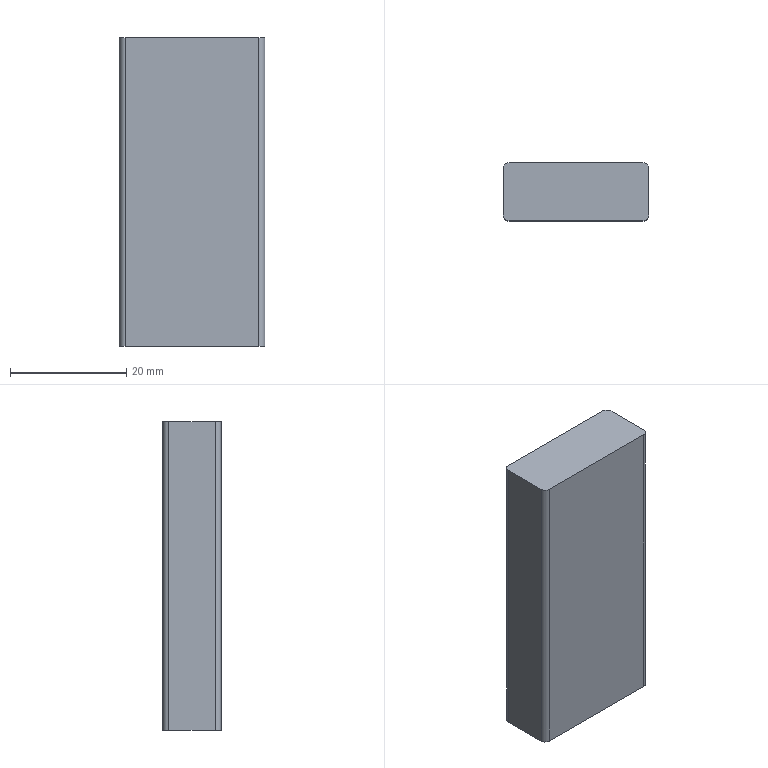Part | STEP file | 200 mesh_id22_xmt | 1 solid | 10 faces | box 24.97 x 9.97 x 53 mm | volume 13149 mm3 | plane 6 | cylinder 4 | commonest cylinder face diameters 2 x4
STEP:
#1=CARTESIAN_POINT('',(-17168.899,-3976.744,0.));
#2=VERTEX_POINT('',#1);
#3=CARTESIAN_POINT('',(-17168.899,-3968.774,0.));
#4=VERTEX_POINT('',#3);
#5=CARTESIAN_POINT('',(-17168.899,-3977.759,0.));
#6=DIRECTION('',(0.,1.,0.));
#7=VECTOR('',#6,1.);
#8=LINE('',#5,#7);
#9=EDGE_CURVE('',#2,#4,#8,.T.);
#10=ORIENTED_EDGE('',*,*,#9,.F.);
#11=CARTESIAN_POINT('',(-17169.899,-3977.744,0.));
#12=VERTEX_POINT('',#11);
#13=CARTESIAN_POINT('',(-17169.899,-3976.744,0.));
#14=DIRECTION('',(0.,0.,-1.));
#15=DIRECTION('',(-1.,0.,0.));
#16=AXIS2_PLACEMENT_3D('',#13,#14,#15);
#17=CIRCLE('',#16,1.);
#18=EDGE_CURVE('',#2,#12,#17,.T.);
#19=ORIENTED_EDGE('',*,*,#18,.T.);
#20=CARTESIAN_POINT('',(-17192.869,-3977.744,0.));
#21=VERTEX_POINT('',#20);
#22=CARTESIAN_POINT('',(-17193.884,-3977.744,0.));
#23=DIRECTION('',(1.,0.,0.));
#24=VECTOR('',#23,1.);
#25=LINE('',#22,#24);
#26=EDGE_CURVE('',#21,#12,#25,.T.);
#27=ORIENTED_EDGE('',*,*,#26,.F.);
#28=CARTESIAN_POINT('',(-17193.869,-3976.744,0.));
#29=VERTEX_POINT('',#28);
#30=CARTESIAN_POINT('',(-17192.869,-3976.744,0.));
#31=DIRECTION('',(0.,0.,-1.));
#32=DIRECTION('',(-1.,0.,0.));
#33=AXIS2_PLACEMENT_3D('',#30,#31,#32);
#34=CIRCLE('',#33,1.);
#35=EDGE_CURVE('',#21,#29,#34,.T.);
#36=ORIENTED_EDGE('',*,*,#35,.T.);
#37=CARTESIAN_POINT('',(-17193.869,-3968.774,0.));
#38=VERTEX_POINT('',#37);
#39=CARTESIAN_POINT('',(-17193.869,-3967.759,0.));
#40=DIRECTION('',(0.,-1.,0.));
#41=VECTOR('',#40,1.);
#42=LINE('',#39,#41);
#43=EDGE_CURVE('',#38,#29,#42,.T.);
#44=ORIENTED_EDGE('',*,*,#43,.F.);
#45=CARTESIAN_POINT('',(-17192.869,-3967.774,0.));
#46=VERTEX_POINT('',#45);
#47=CARTESIAN_POINT('',(-17192.869,-3968.774,0.));
#48=DIRECTION('',(0.,0.,-1.));
#49=DIRECTION('',(-1.,0.,0.));
#50=AXIS2_PLACEMENT_3D('',#47,#48,#49);
#51=CIRCLE('',#50,1.);
#52=EDGE_CURVE('',#38,#46,#51,.T.);
#53=ORIENTED_EDGE('',*,*,#52,.T.);
#54=CARTESIAN_POINT('',(-17169.899,-3967.774,0.));
#55=VERTEX_POINT('',#54);
#56=CARTESIAN_POINT('',(-17168.884,-3967.774,0.));
#57=DIRECTION('',(-1.,0.,0.));
#58=VECTOR('',#57,1.);
#59=LINE('',#56,#58);
#60=EDGE_CURVE('',#55,#46,#59,.T.);
#61=ORIENTED_EDGE('',*,*,#60,.F.);
#62=CARTESIAN_POINT('',(-17169.899,-3968.774,0.));
#63=DIRECTION('',(0.,0.,-1.));
#64=DIRECTION('',(-1.,0.,0.));
#65=AXIS2_PLACEMENT_3D('',#62,#63,#64);
#66=CIRCLE('',#65,1.);
#67=EDGE_CURVE('',#55,#4,#66,.T.);
#68=ORIENTED_EDGE('',*,*,#67,.T.);
#69=EDGE_LOOP('',(#10,#19,#27,#36,#44,#53,#61,#68));
#70=FACE_OUTER_BOUND('',#69,.T.);
#71=CARTESIAN_POINT('',(2237.268,0.00008806,0.));
#72=DIRECTION('',(0.,0.,-1.));
#73=DIRECTION('',(-1.,0.,0.));
#74=AXIS2_PLACEMENT_3D('',#71,#72,#73);
#75=PLANE('',#74);
#76=ADVANCED_FACE('',(#70),#75,.T.);
#77=ORIENTED_EDGE('',*,*,#43,.T.);
#78=CARTESIAN_POINT('',(-17193.869,-3976.744,53.));
#79=VERTEX_POINT('',#78);
#80=CARTESIAN_POINT('',(-17193.869,-3976.744,-382.7));
#81=DIRECTION('',(0.,0.,1.));
#82=VECTOR('',#81,1.);
#83=LINE('',#80,#82);
#84=EDGE_CURVE('',#29,#79,#83,.T.);
#85=ORIENTED_EDGE('',*,*,#84,.T.);
#86=CARTESIAN_POINT('',(-17193.869,-3968.774,53.));
#87=VERTEX_POINT('',#86);
#88=CARTESIAN_POINT('',(-17193.869,0.,53.));
#89=DIRECTION('',(0.,-1.,0.));
#90=VECTOR('',#89,1.);
#91=LINE('',#88,#90);
#92=EDGE_CURVE('',#87,#79,#91,.T.);
#93=ORIENTED_EDGE('',*,*,#92,.F.);
#94=CARTESIAN_POINT('',(-17193.869,-3968.774,-382.7));
#95=DIRECTION('',(0.,0.,-1.));
#96=VECTOR('',#95,1.);
#97=LINE('',#94,#96);
#98=EDGE_CURVE('',#87,#38,#97,.T.);
#99=ORIENTED_EDGE('',*,*,#98,.T.);
#100=EDGE_LOOP('',(#77,#85,#93,#99));
#101=FACE_OUTER_BOUND('',#100,.T.);
#102=CARTESIAN_POINT('',(-17193.869,-3967.759,-382.7));
#103=DIRECTION('',(-1.,0.,0.));
#104=DIRECTION('',(0.,0.,1.));
#105=AXIS2_PLACEMENT_3D('',#102,#103,#104);
#106=PLANE('',#105);
#107=ADVANCED_FACE('',(#101),#106,.T.);
#108=CARTESIAN_POINT('',(-17192.869,-3977.744,53.));
#109=VERTEX_POINT('',#108);
#110=CARTESIAN_POINT('',(-17169.899,-3977.744,53.));
#111=VERTEX_POINT('',#110);
#112=CARTESIAN_POINT('',(0.,-3977.744,53.));
#113=DIRECTION('',(1.,0.,0.));
#114=VECTOR('',#113,1.);
#115=LINE('',#112,#114);
#116=EDGE_CURVE('',#109,#111,#115,.T.);
#117=ORIENTED_EDGE('',*,*,#116,.T.);
#118=CARTESIAN_POINT('',(-17168.899,-3976.744,53.));
#119=VERTEX_POINT('',#118);
#120=CARTESIAN_POINT('',(-17169.899,-3976.744,53.));
#121=DIRECTION('',(0.,0.,1.));
#122=DIRECTION('',(1.,0.,0.));
#123=AXIS2_PLACEMENT_3D('',#120,#121,#122);
#124=CIRCLE('',#123,1.);
#125=EDGE_CURVE('',#111,#119,#124,.T.);
#126=ORIENTED_EDGE('',*,*,#125,.T.);
#127=CARTESIAN_POINT('',(-17168.899,-3968.774,53.));
#128=VERTEX_POINT('',#127);
#129=CARTESIAN_POINT('',(-17168.899,0.,53.));
#130=DIRECTION('',(0.,1.,0.));
#131=VECTOR('',#130,1.);
#132=LINE('',#129,#131);
#133=EDGE_CURVE('',#119,#128,#132,.T.);
#134=ORIENTED_EDGE('',*,*,#133,.T.);
#135=CARTESIAN_POINT('',(-17169.899,-3967.774,53.));
#136=VERTEX_POINT('',#135);
#137=CARTESIAN_POINT('',(-17169.899,-3968.774,53.));
#138=DIRECTION('',(0.,0.,1.));
#139=DIRECTION('',(1.,0.,0.));
#140=AXIS2_PLACEMENT_3D('',#137,#138,#139);
#141=CIRCLE('',#140,1.);
#142=EDGE_CURVE('',#128,#136,#141,.T.);
#143=ORIENTED_EDGE('',*,*,#142,.T.);
#144=CARTESIAN_POINT('',(-17192.869,-3967.774,53.));
#145=VERTEX_POINT('',#144);
#146=CARTESIAN_POINT('',(0.,-3967.774,53.));
#147=DIRECTION('',(-1.,0.,0.));
#148=VECTOR('',#147,1.);
#149=LINE('',#146,#148);
#150=EDGE_CURVE('',#136,#145,#149,.T.);
#151=ORIENTED_EDGE('',*,*,#150,.T.);
#152=CARTESIAN_POINT('',(-17192.869,-3968.774,53.));
#153=DIRECTION('',(0.,0.,1.));
#154=DIRECTION('',(1.,0.,0.));
#155=AXIS2_PLACEMENT_3D('',#152,#153,#154);
#156=CIRCLE('',#155,1.);
#157=EDGE_CURVE('',#145,#87,#156,.T.);
#158=ORIENTED_EDGE('',*,*,#157,.T.);
#159=ORIENTED_EDGE('',*,*,#92,.T.);
#160=CARTESIAN_POINT('',(-17192.869,-3976.744,53.));
#161=DIRECTION('',(0.,0.,1.));
#162=DIRECTION('',(1.,0.,0.));
#163=AXIS2_PLACEMENT_3D('',#160,#161,#162);
#164=CIRCLE('',#163,1.);
#165=EDGE_CURVE('',#79,#109,#164,.T.);
#166=ORIENTED_EDGE('',*,*,#165,.T.);
#167=EDGE_LOOP('',(#117,#126,#134,#143,#151,#158,#159,#166));
#168=FACE_OUTER_BOUND('',#167,.T.);
#169=CARTESIAN_POINT('',(0.,0.,53.));
#170=DIRECTION('',(0.,0.,1.));
#171=DIRECTION('',(1.,0.,0.));
#172=AXIS2_PLACEMENT_3D('',#169,#170,#171);
#173=PLANE('',#172);
#174=ADVANCED_FACE('',(#168),#173,.T.);
#175=ORIENTED_EDGE('',*,*,#60,.T.);
#176=CARTESIAN_POINT('',(-17192.869,-3967.774,-382.7));
#177=DIRECTION('',(0.,0.,1.));
#178=VECTOR('',#177,1.);
#179=LINE('',#176,#178);
#180=EDGE_CURVE('',#46,#145,#179,.T.);
#181=ORIENTED_EDGE('',*,*,#180,.T.);
#182=ORIENTED_EDGE('',*,*,#150,.F.);
#183=CARTESIAN_POINT('',(-17169.899,-3967.774,-382.7));
#184=DIRECTION('',(0.,0.,-1.));
#185=VECTOR('',#184,1.);
#186=LINE('',#183,#185);
#187=EDGE_CURVE('',#136,#55,#186,.T.);
#188=ORIENTED_EDGE('',*,*,#187,.T.);
#189=EDGE_LOOP('',(#175,#181,#182,#188));
#190=FACE_OUTER_BOUND('',#189,.T.);
#191=CARTESIAN_POINT('',(-17168.884,-3967.774,-382.7));
#192=DIRECTION('',(0.,1.,0.));
#193=DIRECTION('',(0.,0.,1.));
#194=AXIS2_PLACEMENT_3D('',#191,#192,#193);
#195=PLANE('',#194);
#196=ADVANCED_FACE('',(#190),#195,.T.);
#197=ORIENTED_EDGE('',*,*,#26,.T.);
#198=CARTESIAN_POINT('',(-17169.899,-3977.744,-382.7));
#199=DIRECTION('',(0.,0.,1.));
#200=VECTOR('',#199,1.);
#201=LINE('',#198,#200);
#202=EDGE_CURVE('',#12,#111,#201,.T.);
#203=ORIENTED_EDGE('',*,*,#202,.T.);
#204=ORIENTED_EDGE('',*,*,#116,.F.);
#205=CARTESIAN_POINT('',(-17192.869,-3977.744,-382.7));
#206=DIRECTION('',(0.,0.,-1.));
#207=VECTOR('',#206,1.);
#208=LINE('',#205,#207);
#209=EDGE_CURVE('',#109,#21,#208,.T.);
#210=ORIENTED_EDGE('',*,*,#209,.T.);
#211=EDGE_LOOP('',(#197,#203,#204,#210));
#212=FACE_OUTER_BOUND('',#211,.T.);
#213=CARTESIAN_POINT('',(-17193.884,-3977.744,-382.7));
#214=DIRECTION('',(0.,-1.,0.));
#215=DIRECTION('',(0.,0.,-1.));
#216=AXIS2_PLACEMENT_3D('',#213,#214,#215);
#217=PLANE('',#216);
#218=ADVANCED_FACE('',(#212),#217,.T.);
#219=ORIENTED_EDGE('',*,*,#133,.F.);
#220=CARTESIAN_POINT('',(-17168.899,-3976.744,-382.7));
#221=DIRECTION('',(0.,0.,-1.));
#222=VECTOR('',#221,1.);
#223=LINE('',#220,#222);
#224=EDGE_CURVE('',#119,#2,#223,.T.);
#225=ORIENTED_EDGE('',*,*,#224,.T.);
#226=ORIENTED_EDGE('',*,*,#9,.T.);
#227=CARTESIAN_POINT('',(-17168.899,-3968.774,-382.7));
#228=DIRECTION('',(0.,0.,1.));
#229=VECTOR('',#228,1.);
#230=LINE('',#227,#229);
#231=EDGE_CURVE('',#4,#128,#230,.T.);
#232=ORIENTED_EDGE('',*,*,#231,.T.);
#233=EDGE_LOOP('',(#219,#225,#226,#232));
#234=FACE_OUTER_BOUND('',#233,.T.);
#235=CARTESIAN_POINT('',(-17168.899,-3977.759,-382.7));
#236=DIRECTION('',(1.,0.,0.));
#237=DIRECTION('',(0.,0.,-1.));
#238=AXIS2_PLACEMENT_3D('',#235,#236,#237);
#239=PLANE('',#238);
#240=ADVANCED_FACE('',(#234),#239,.T.);
#241=ORIENTED_EDGE('',*,*,#18,.F.);
#242=ORIENTED_EDGE('',*,*,#224,.F.);
#243=ORIENTED_EDGE('',*,*,#125,.F.);
#244=ORIENTED_EDGE('',*,*,#202,.F.);
#245=EDGE_LOOP('',(#241,#242,#243,#244));
#246=FACE_OUTER_BOUND('',#245,.T.);
#247=CARTESIAN_POINT('',(-17169.899,-3976.744,-382.7));
#248=DIRECTION('',(0.,0.,1.));
#249=DIRECTION('',(1.,0.,0.));
#250=AXIS2_PLACEMENT_3D('',#247,#248,#249);
#251=CYLINDRICAL_SURFACE('',#250,1.);
#252=ADVANCED_FACE('',(#246),#251,.T.);
#253=ORIENTED_EDGE('',*,*,#35,.F.);
#254=ORIENTED_EDGE('',*,*,#209,.F.);
#255=ORIENTED_EDGE('',*,*,#165,.F.);
#256=ORIENTED_EDGE('',*,*,#84,.F.);
#257=EDGE_LOOP('',(#253,#254,#255,#256));
#258=FACE_OUTER_BOUND('',#257,.T.);
#259=CARTESIAN_POINT('',(-17192.869,-3976.744,-382.7));
#260=DIRECTION('',(0.,0.,1.));
#261=DIRECTION('',(1.,0.,0.));
#262=AXIS2_PLACEMENT_3D('',#259,#260,#261);
#263=CYLINDRICAL_SURFACE('',#262,1.);
#264=ADVANCED_FACE('',(#258),#263,.T.);
#265=ORIENTED_EDGE('',*,*,#52,.F.);
#266=ORIENTED_EDGE('',*,*,#98,.F.);
#267=ORIENTED_EDGE('',*,*,#157,.F.);
#268=ORIENTED_EDGE('',*,*,#180,.F.);
#269=EDGE_LOOP('',(#265,#266,#267,#268));
#270=FACE_OUTER_BOUND('',#269,.T.);
#271=CARTESIAN_POINT('',(-17192.869,-3968.774,-382.7));
#272=DIRECTION('',(0.,0.,1.));
#273=DIRECTION('',(1.,0.,0.));
#274=AXIS2_PLACEMENT_3D('',#271,#272,#273);
#275=CYLINDRICAL_SURFACE('',#274,1.);
#276=ADVANCED_FACE('',(#270),#275,.T.);
#277=ORIENTED_EDGE('',*,*,#67,.F.);
#278=ORIENTED_EDGE('',*,*,#187,.F.);
#279=ORIENTED_EDGE('',*,*,#142,.F.);
#280=ORIENTED_EDGE('',*,*,#231,.F.);
#281=EDGE_LOOP('',(#277,#278,#279,#280));
#282=FACE_OUTER_BOUND('',#281,.T.);
#283=CARTESIAN_POINT('',(-17169.899,-3968.774,-382.7));
#284=DIRECTION('',(0.,0.,1.));
#285=DIRECTION('',(1.,0.,0.));
#286=AXIS2_PLACEMENT_3D('',#283,#284,#285);
#287=CYLINDRICAL_SURFACE('',#286,1.);
#288=ADVANCED_FACE('',(#282),#287,.T.);
#289=CLOSED_SHELL('',(#76,#107,#174,#196,#218,#240,#252,#264,#276,#288));
#290=MANIFOLD_SOLID_BREP('',#289);
#291=(LENGTH_UNIT()NAMED_UNIT(*)SI_UNIT(.MILLI.,.METRE.));
#292=UNCERTAINTY_MEASURE_WITH_UNIT(LENGTH_MEASURE(0.00002),#291,'','');
#293=(NAMED_UNIT(*)PLANE_ANGLE_UNIT()SI_UNIT($,.RADIAN.));
#294=PLANE_ANGLE_MEASURE_WITH_UNIT(PLANE_ANGLE_MEASURE(0.01745),#293);
#295=DIMENSIONAL_EXPONENTS(0.,0.,0.,0.,0.,0.,0.);
#296=(CONVERSION_BASED_UNIT('DEGREE',#294)NAMED_UNIT(#295)PLANE_ANGLE_UNIT());
#297=(NAMED_UNIT(*)SI_UNIT($,.STERADIAN.)SOLID_ANGLE_UNIT());
#298=(GEOMETRIC_REPRESENTATION_CONTEXT(3)GLOBAL_UNCERTAINTY_ASSIGNED_CONTEXT((#292))GLOBAL_UNIT_ASSIGNED_CONTEXT((#291,#296,#297))REPRESENTATION_CONTEXT('',''));
#299=ADVANCED_BREP_SHAPE_REPRESENTATION('',(#290),#298);